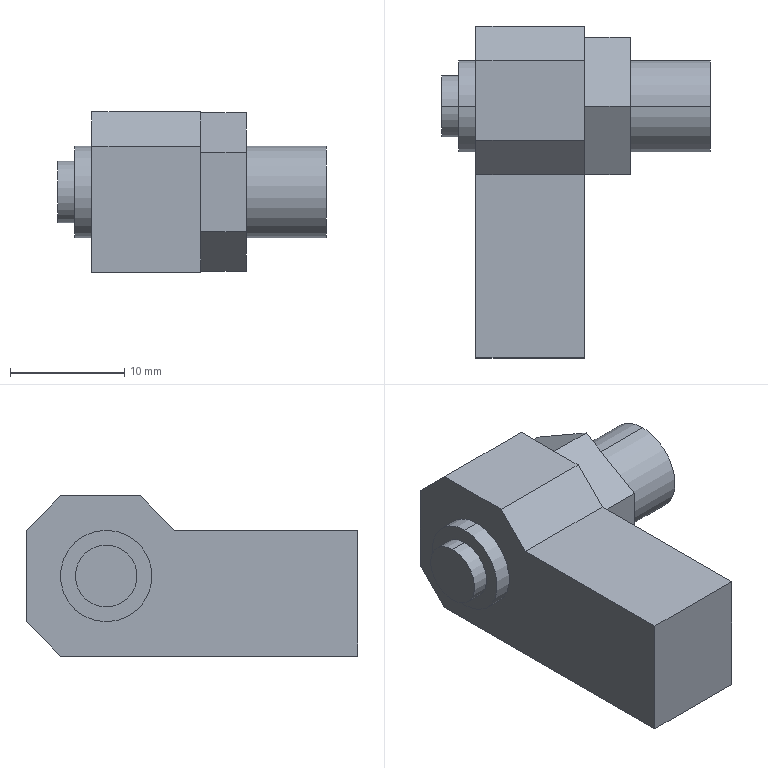Part | STEP file | 0246_Z_102_MXQ12L-30AS-A93_3 | 1 solid | 59 faces | box 23.5 x 29 x 14 mm | volume 4066 mm3 | plane 45 | cylinder 14 | commonest cylinder face diameters 7 x4 7.5 x4 8 x4 5.4 x2